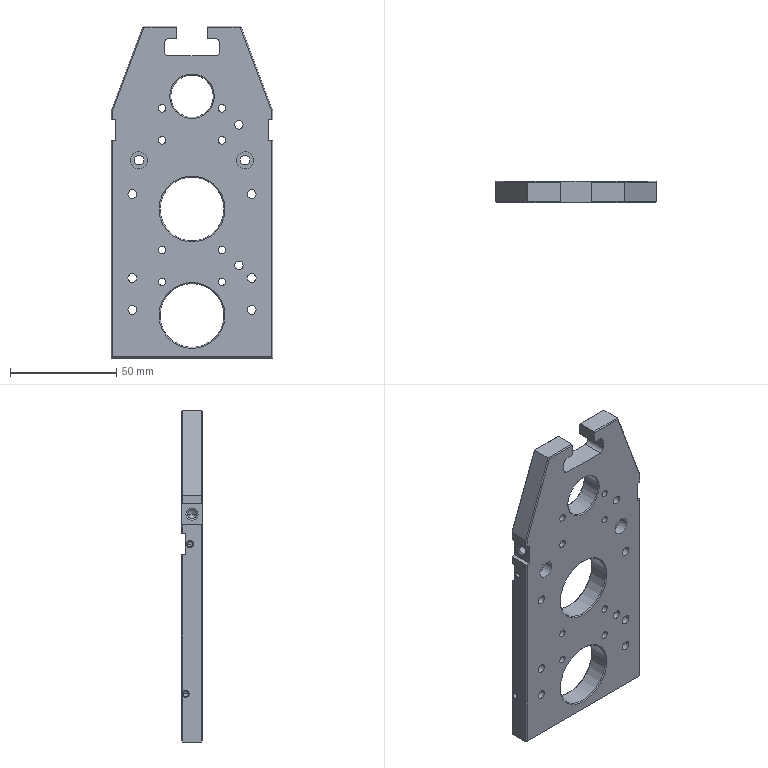Part | NX | 1 solid | 182 faces | box 76 x 10 x 156 mm | volume 86757 mm3 | cylinder 78 | plane 60 | cone 44 | commonest cylinder face diameters 3.5 x16 4.2 x16 6 x16 2.5 x8 4 x8 4.5 x4